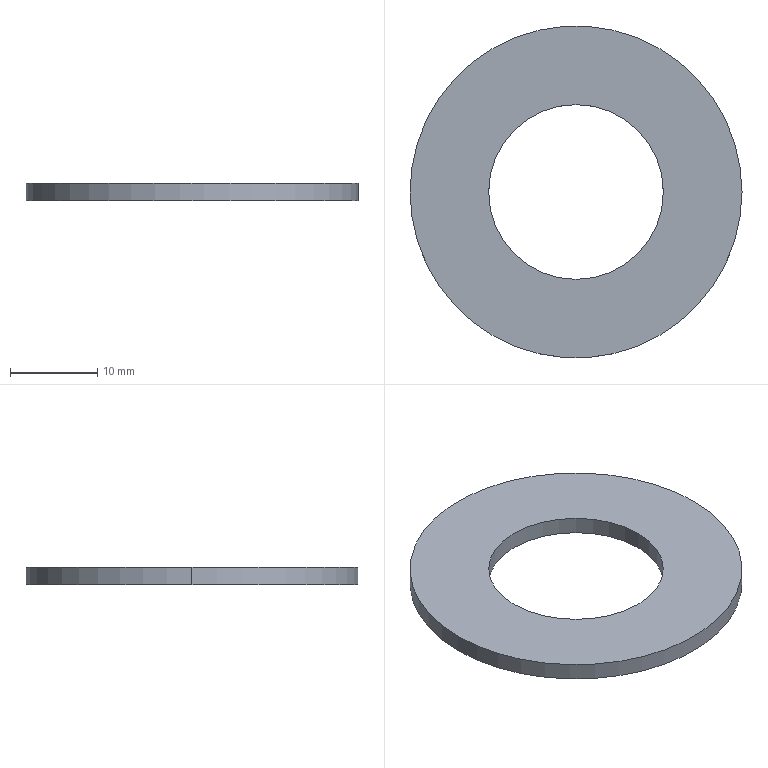Part | NX | 1 solid | 6 faces | box 38 x 38 x 2 mm | volume 1640 mm3 | cylinder 4 | plane 2 | commonest cylinder face diameters 20 x2 38 x2
STEP:
#1=CARTESIAN_POINT('',(19.,0.,0.));
#2=VERTEX_POINT('',#1);
#3=CARTESIAN_POINT('',(-19.,0.,0.));
#4=VERTEX_POINT('',#3);
#5=CARTESIAN_POINT('',(0.,0.,0.));
#6=DIRECTION('',(0.,0.,1.));
#7=DIRECTION('',(-1.,0.,0.));
#8=AXIS2_PLACEMENT_3D('',#5,#6,#7);
#9=CIRCLE('',#8,19.);
#10=EDGE_CURVE('',#2,#4,#9,.T.);
#11=ORIENTED_EDGE('',*,*,#10,.F.);
#12=CARTESIAN_POINT('',(0.,0.,0.));
#13=DIRECTION('',(0.,0.,1.));
#14=DIRECTION('',(-1.,0.,0.));
#15=AXIS2_PLACEMENT_3D('',#12,#13,#14);
#16=CIRCLE('',#15,19.);
#17=EDGE_CURVE('',#4,#2,#16,.T.);
#18=ORIENTED_EDGE('',*,*,#17,.F.);
#19=EDGE_LOOP('',(#11,#18));
#20=FACE_BOUND('',#19,.T.);
#21=CARTESIAN_POINT('',(-10.,0.,0.));
#22=VERTEX_POINT('',#21);
#23=CARTESIAN_POINT('',(10.,0.,0.));
#24=VERTEX_POINT('',#23);
#25=CARTESIAN_POINT('',(0.,0.,0.));
#26=DIRECTION('',(0.,0.,-1.));
#27=DIRECTION('',(-1.,0.,0.));
#28=AXIS2_PLACEMENT_3D('',#25,#26,#27);
#29=CIRCLE('',#28,10.);
#30=EDGE_CURVE('',#22,#24,#29,.T.);
#31=ORIENTED_EDGE('',*,*,#30,.F.);
#32=CARTESIAN_POINT('',(0.,0.,0.));
#33=DIRECTION('',(0.,0.,-1.));
#34=DIRECTION('',(-1.,0.,0.));
#35=AXIS2_PLACEMENT_3D('',#32,#33,#34);
#36=CIRCLE('',#35,10.);
#37=EDGE_CURVE('',#24,#22,#36,.T.);
#38=ORIENTED_EDGE('',*,*,#37,.F.);
#39=EDGE_LOOP('',(#31,#38));
#40=FACE_BOUND('',#39,.T.);
#41=CARTESIAN_POINT('',(0.,0.,0.));
#42=DIRECTION('',(0.,0.,1.));
#43=DIRECTION('',(1.,0.,0.));
#44=AXIS2_PLACEMENT_3D('',#41,#42,#43);
#45=PLANE('',#44);
#46=ADVANCED_FACE('',(#20,#40),#45,.F.);
#47=CARTESIAN_POINT('',(19.,0.,2.));
#48=VERTEX_POINT('',#47);
#49=CARTESIAN_POINT('',(-19.,0.,2.));
#50=VERTEX_POINT('',#49);
#51=CARTESIAN_POINT('',(0.,0.,2.));
#52=DIRECTION('',(0.,0.,-1.));
#53=DIRECTION('',(1.,0.,0.));
#54=AXIS2_PLACEMENT_3D('',#51,#52,#53);
#55=CIRCLE('',#54,19.);
#56=EDGE_CURVE('',#48,#50,#55,.T.);
#57=ORIENTED_EDGE('',*,*,#56,.T.);
#58=CARTESIAN_POINT('',(-19.,0.,0.));
#59=DIRECTION('',(0.,0.,1.));
#60=VECTOR('',#59,1000.);
#61=LINE('',#58,#60);
#62=EDGE_CURVE('',#50,#4,#61,.F.);
#63=ORIENTED_EDGE('',*,*,#62,.T.);
#64=ORIENTED_EDGE('',*,*,#17,.T.);
#65=CARTESIAN_POINT('',(19.,0.,0.));
#66=DIRECTION('',(0.,0.,1.));
#67=VECTOR('',#66,1000.);
#68=LINE('',#65,#67);
#69=EDGE_CURVE('',#48,#2,#68,.F.);
#70=ORIENTED_EDGE('',*,*,#69,.F.);
#71=EDGE_LOOP('',(#57,#63,#64,#70));
#72=FACE_BOUND('',#71,.T.);
#73=CARTESIAN_POINT('',(0.,0.,0.));
#74=DIRECTION('',(0.,0.,1.));
#75=DIRECTION('',(1.,0.,0.));
#76=AXIS2_PLACEMENT_3D('',#73,#74,#75);
#77=CYLINDRICAL_SURFACE('',#76,19.);
#78=ADVANCED_FACE('',(#72),#77,.T.);
#79=CARTESIAN_POINT('',(-10.,0.,2.));
#80=VERTEX_POINT('',#79);
#81=CARTESIAN_POINT('',(10.,0.,2.));
#82=VERTEX_POINT('',#81);
#83=CARTESIAN_POINT('',(0.,0.,2.));
#84=DIRECTION('',(0.,0.,1.));
#85=DIRECTION('',(1.,0.,0.));
#86=AXIS2_PLACEMENT_3D('',#83,#84,#85);
#87=CIRCLE('',#86,10.);
#88=EDGE_CURVE('',#80,#82,#87,.T.);
#89=ORIENTED_EDGE('',*,*,#88,.T.);
#90=CARTESIAN_POINT('',(10.,0.,0.));
#91=DIRECTION('',(0.,0.,1.));
#92=VECTOR('',#91,1000.);
#93=LINE('',#90,#92);
#94=EDGE_CURVE('',#24,#82,#93,.T.);
#95=ORIENTED_EDGE('',*,*,#94,.F.);
#96=ORIENTED_EDGE('',*,*,#37,.T.);
#97=CARTESIAN_POINT('',(-10.,0.,0.));
#98=DIRECTION('',(0.,0.,1.));
#99=VECTOR('',#98,1000.);
#100=LINE('',#97,#99);
#101=EDGE_CURVE('',#22,#80,#100,.T.);
#102=ORIENTED_EDGE('',*,*,#101,.T.);
#103=EDGE_LOOP('',(#89,#95,#96,#102));
#104=FACE_BOUND('',#103,.T.);
#105=CARTESIAN_POINT('',(0.,0.,0.));
#106=DIRECTION('',(0.,0.,1.));
#107=DIRECTION('',(1.,0.,0.));
#108=AXIS2_PLACEMENT_3D('',#105,#106,#107);
#109=CYLINDRICAL_SURFACE('',#108,10.);
#110=ADVANCED_FACE('',(#104),#109,.F.);
#111=ORIENTED_EDGE('',*,*,#56,.F.);
#112=CARTESIAN_POINT('',(0.,0.,2.));
#113=DIRECTION('',(0.,0.,-1.));
#114=DIRECTION('',(1.,0.,0.));
#115=AXIS2_PLACEMENT_3D('',#112,#113,#114);
#116=CIRCLE('',#115,19.);
#117=EDGE_CURVE('',#50,#48,#116,.T.);
#118=ORIENTED_EDGE('',*,*,#117,.F.);
#119=EDGE_LOOP('',(#111,#118));
#120=FACE_BOUND('',#119,.T.);
#121=ORIENTED_EDGE('',*,*,#88,.F.);
#122=CARTESIAN_POINT('',(0.,0.,2.));
#123=DIRECTION('',(0.,0.,1.));
#124=DIRECTION('',(1.,0.,0.));
#125=AXIS2_PLACEMENT_3D('',#122,#123,#124);
#126=CIRCLE('',#125,10.);
#127=EDGE_CURVE('',#82,#80,#126,.T.);
#128=ORIENTED_EDGE('',*,*,#127,.F.);
#129=EDGE_LOOP('',(#121,#128));
#130=FACE_BOUND('',#129,.T.);
#131=CARTESIAN_POINT('',(0.,0.,2.));
#132=DIRECTION('',(0.,0.,1.));
#133=DIRECTION('',(1.,0.,0.));
#134=AXIS2_PLACEMENT_3D('',#131,#132,#133);
#135=PLANE('',#134);
#136=ADVANCED_FACE('',(#120,#130),#135,.T.);
#137=ORIENTED_EDGE('',*,*,#10,.T.);
#138=ORIENTED_EDGE('',*,*,#62,.F.);
#139=ORIENTED_EDGE('',*,*,#117,.T.);
#140=ORIENTED_EDGE('',*,*,#69,.T.);
#141=EDGE_LOOP('',(#137,#138,#139,#140));
#142=FACE_BOUND('',#141,.T.);
#143=CARTESIAN_POINT('',(0.,0.,0.));
#144=DIRECTION('',(0.,0.,1.));
#145=DIRECTION('',(1.,0.,0.));
#146=AXIS2_PLACEMENT_3D('',#143,#144,#145);
#147=CYLINDRICAL_SURFACE('',#146,19.);
#148=ADVANCED_FACE('',(#142),#147,.T.);
#149=ORIENTED_EDGE('',*,*,#30,.T.);
#150=ORIENTED_EDGE('',*,*,#94,.T.);
#151=ORIENTED_EDGE('',*,*,#127,.T.);
#152=ORIENTED_EDGE('',*,*,#101,.F.);
#153=EDGE_LOOP('',(#149,#150,#151,#152));
#154=FACE_BOUND('',#153,.T.);
#155=CARTESIAN_POINT('',(0.,0.,0.));
#156=DIRECTION('',(0.,0.,1.));
#157=DIRECTION('',(1.,0.,0.));
#158=AXIS2_PLACEMENT_3D('',#155,#156,#157);
#159=CYLINDRICAL_SURFACE('',#158,10.);
#160=ADVANCED_FACE('',(#154),#159,.F.);
#161=CLOSED_SHELL('',(#46,#78,#110,#136,#148,#160));
#162=MANIFOLD_SOLID_BREP('',#161);
#163=(LENGTH_UNIT()NAMED_UNIT(*)SI_UNIT(.MILLI.,.METRE.));
#164=UNCERTAINTY_MEASURE_WITH_UNIT(LENGTH_MEASURE(0.00001),#163,'','');
#165=(NAMED_UNIT(*)PLANE_ANGLE_UNIT()SI_UNIT($,.RADIAN.));
#166=(NAMED_UNIT(*)SI_UNIT($,.STERADIAN.)SOLID_ANGLE_UNIT());
#167=(GEOMETRIC_REPRESENTATION_CONTEXT(3)GLOBAL_UNCERTAINTY_ASSIGNED_CONTEXT((#164))GLOBAL_UNIT_ASSIGNED_CONTEXT((#163,#165,#166))REPRESENTATION_CONTEXT('',''));
#168=ADVANCED_BREP_SHAPE_REPRESENTATION('',(#162),#167);